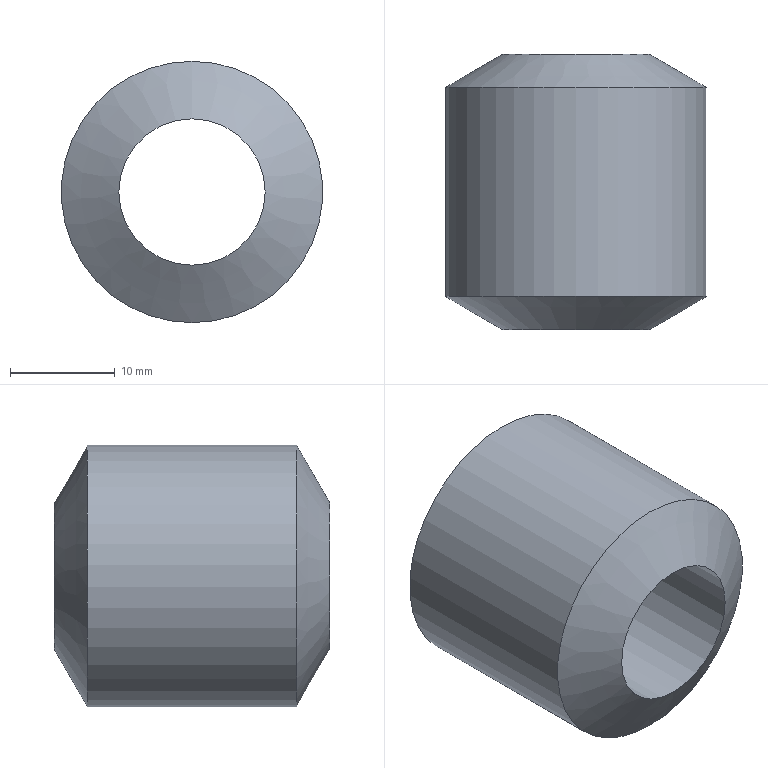Part | NX | features DATUM_CSYS 4, SKETCH 3, EXTRACT_DATUM_AXIS 2, EXTRACT_DATUM_PLANE 2, EXTRACT_FACE 2, EXTRACT_STRING 2, SWP104 2, EXTRUDE 1, Instance Feature 1, Mirror Feature 1 | 1 solid | 4 faces | box 25 x 26.35 x 25 mm | volume 7708 mm3 | cylinder 2 | cone 2 | commonest cylinder face diameters 14 x1 25 x1
STEP:
#1=CARTESIAN_POINT('',(0.,-10.,12.5));
#2=VERTEX_POINT('',#1);
#3=CARTESIAN_POINT('',(0.,-10.,0.));
#4=DIRECTION('',(0.,1.,0.));
#5=DIRECTION('',(0.,0.,1.));
#6=AXIS2_PLACEMENT_3D('',#3,#4,#5);
#7=CIRCLE('',#6,12.5);
#8=EDGE_CURVE('',#2,#2,#7,.T.);
#9=ORIENTED_EDGE('',*,*,#8,.T.);
#10=EDGE_LOOP('',(#9));
#11=FACE_BOUND('',#10,.T.);
#12=CARTESIAN_POINT('',(0.,10.,-12.5));
#13=VERTEX_POINT('',#12);
#14=CARTESIAN_POINT('',(0.,10.,0.));
#15=DIRECTION('',(0.,-1.,0.));
#16=DIRECTION('',(0.,0.,-1.));
#17=AXIS2_PLACEMENT_3D('',#14,#15,#16);
#18=CIRCLE('',#17,12.5);
#19=EDGE_CURVE('',#13,#13,#18,.T.);
#20=ORIENTED_EDGE('',*,*,#19,.T.);
#21=EDGE_LOOP('',(#20));
#22=FACE_BOUND('',#21,.T.);
#23=CARTESIAN_POINT('',(0.,-13.175,0.));
#24=DIRECTION('',(0.,1.,0.));
#25=DIRECTION('',(0.,0.,1.));
#26=AXIS2_PLACEMENT_3D('',#23,#24,#25);
#27=CYLINDRICAL_SURFACE('',#26,12.5);
#28=ADVANCED_FACE('',(#11,#22),#27,.T.);
#29=CARTESIAN_POINT('',(0.,-13.175,7.));
#30=VERTEX_POINT('',#29);
#31=CARTESIAN_POINT('',(0.,-13.175,0.));
#32=DIRECTION('',(0.,1.,0.));
#33=DIRECTION('',(0.,0.,1.));
#34=AXIS2_PLACEMENT_3D('',#31,#32,#33);
#35=CIRCLE('',#34,7.);
#36=EDGE_CURVE('',#30,#30,#35,.T.);
#37=ORIENTED_EDGE('',*,*,#36,.F.);
#38=EDGE_LOOP('',(#37));
#39=FACE_BOUND('',#38,.T.);
#40=CARTESIAN_POINT('',(0.,13.175,-7.));
#41=VERTEX_POINT('',#40);
#42=CARTESIAN_POINT('',(0.,13.175,0.));
#43=DIRECTION('',(0.,-1.,0.));
#44=DIRECTION('',(0.,0.,-1.));
#45=AXIS2_PLACEMENT_3D('',#42,#43,#44);
#46=CIRCLE('',#45,7.);
#47=EDGE_CURVE('',#41,#41,#46,.T.);
#48=ORIENTED_EDGE('',*,*,#47,.F.);
#49=EDGE_LOOP('',(#48));
#50=FACE_BOUND('',#49,.T.);
#51=CARTESIAN_POINT('',(0.,-13.175,0.));
#52=DIRECTION('',(0.,1.,0.));
#53=DIRECTION('',(0.,0.,1.));
#54=AXIS2_PLACEMENT_3D('',#51,#52,#53);
#55=CYLINDRICAL_SURFACE('',#54,7.);
#56=ADVANCED_FACE('',(#39,#50),#55,.F.);
#57=ORIENTED_EDGE('',*,*,#47,.T.);
#58=EDGE_LOOP('',(#57));
#59=FACE_BOUND('',#58,.T.);
#60=ORIENTED_EDGE('',*,*,#19,.F.);
#61=EDGE_LOOP('',(#60));
#62=FACE_BOUND('',#61,.T.);
#63=CARTESIAN_POINT('',(0.,13.175,0.));
#64=DIRECTION('',(0.,-1.,0.));
#65=DIRECTION('',(0.,0.,-1.));
#66=AXIS2_PLACEMENT_3D('',#63,#64,#65);
#67=CONICAL_SURFACE('',#66,7.,1.047);
#68=ADVANCED_FACE('',(#59,#62),#67,.T.);
#69=ORIENTED_EDGE('',*,*,#36,.T.);
#70=EDGE_LOOP('',(#69));
#71=FACE_BOUND('',#70,.T.);
#72=ORIENTED_EDGE('',*,*,#8,.F.);
#73=EDGE_LOOP('',(#72));
#74=FACE_BOUND('',#73,.T.);
#75=CARTESIAN_POINT('',(0.,-13.175,0.));
#76=DIRECTION('',(0.,1.,0.));
#77=DIRECTION('',(0.,0.,1.));
#78=AXIS2_PLACEMENT_3D('',#75,#76,#77);
#79=CONICAL_SURFACE('',#78,7.,1.047);
#80=ADVANCED_FACE('',(#71,#74),#79,.T.);
#81=CLOSED_SHELL('',(#28,#56,#68,#80));
#82=MANIFOLD_SOLID_BREP('',#81);
#83=(LENGTH_UNIT()NAMED_UNIT(*)SI_UNIT(.MILLI.,.METRE.));
#84=UNCERTAINTY_MEASURE_WITH_UNIT(LENGTH_MEASURE(0.00001),#83,'','');
#85=(NAMED_UNIT(*)PLANE_ANGLE_UNIT()SI_UNIT($,.RADIAN.));
#86=(NAMED_UNIT(*)SI_UNIT($,.STERADIAN.)SOLID_ANGLE_UNIT());
#87=(GEOMETRIC_REPRESENTATION_CONTEXT(3)GLOBAL_UNCERTAINTY_ASSIGNED_CONTEXT((#84))GLOBAL_UNIT_ASSIGNED_CONTEXT((#83,#85,#86))REPRESENTATION_CONTEXT('',''));
#88=ADVANCED_BREP_SHAPE_REPRESENTATION('',(#82),#87);